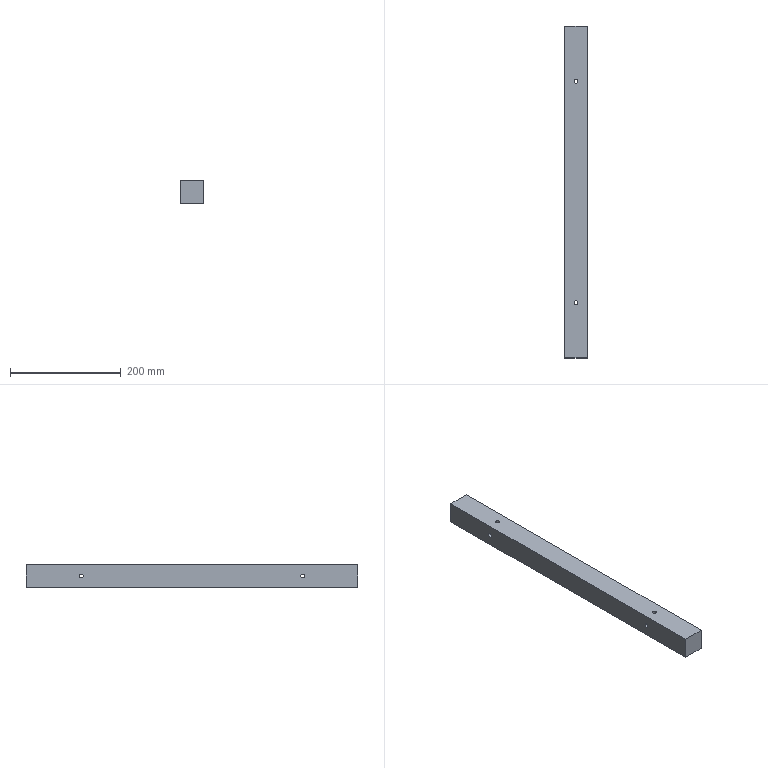Part | NX | features 切除-拉伸3[1] 2 | 1 solid | 22 faces | box 40 x 600 x 40 mm | volume 954300 mm3 | cylinder 16 | plane 6 | commonest cylinder face diameters 7 x16
STEP:
#1=CARTESIAN_POINT('',(-127.,-500.,3.515));
#2=VERTEX_POINT('',#1);
#3=CARTESIAN_POINT('',(-143.5,-500.,3.515));
#4=VERTEX_POINT('',#3);
#5=CARTESIAN_POINT('',(1333.,-500.,3.515));
#6=DIRECTION('',(-1.,0.,0.));
#7=VECTOR('',#6,1000.);
#8=LINE('',#5,#7);
#9=EDGE_CURVE('',#2,#4,#8,.T.);
#10=ORIENTED_EDGE('',*,*,#9,.F.);
#11=CARTESIAN_POINT('',(-127.,-500.,10.515));
#12=VERTEX_POINT('',#11);
#13=CARTESIAN_POINT('',(-127.,-500.,7.015));
#14=DIRECTION('',(1.,0.,0.));
#15=DIRECTION('',(0.,0.,-1.));
#16=AXIS2_PLACEMENT_3D('',#13,#14,#15);
#17=CIRCLE('',#16,3.5);
#18=EDGE_CURVE('',#2,#12,#17,.T.);
#19=ORIENTED_EDGE('',*,*,#18,.T.);
#20=CARTESIAN_POINT('',(-143.5,-500.,10.515));
#21=VERTEX_POINT('',#20);
#22=CARTESIAN_POINT('',(1333.,-500.,10.515));
#23=DIRECTION('',(-1.,0.,0.));
#24=VECTOR('',#23,1000.);
#25=LINE('',#22,#24);
#26=EDGE_CURVE('',#21,#12,#25,.F.);
#27=ORIENTED_EDGE('',*,*,#26,.F.);
#28=CARTESIAN_POINT('',(-147.,-496.5,7.015));
#29=VERTEX_POINT('',#28);
#30=CARTESIAN_POINT('',(-147.,-496.5,7.015));
#31=CARTESIAN_POINT('',(-144.95,-496.5,9.066));
#32=CARTESIAN_POINT('',(-143.5,-497.95,10.515));
#33=CARTESIAN_POINT('',(-143.5,-500.,10.515));
#34=(BOUNDED_CURVE()B_SPLINE_CURVE(3,(#30,#31,#32,#33),.UNSPECIFIED.,.F.,.F.)B_SPLINE_CURVE_WITH_KNOTS((4,4),(4.712,6.283),.UNSPECIFIED.)CURVE()GEOMETRIC_REPRESENTATION_ITEM()RATIONAL_B_SPLINE_CURVE((1.,0.8047,0.8047,1.))REPRESENTATION_ITEM(''));
#35=EDGE_CURVE('',#29,#21,#34,.T.);
#36=ORIENTED_EDGE('',*,*,#35,.F.);
#37=CARTESIAN_POINT('',(-143.5,-500.,3.515));
#38=CARTESIAN_POINT('',(-143.5,-497.95,3.515));
#39=CARTESIAN_POINT('',(-144.95,-496.5,4.965));
#40=CARTESIAN_POINT('',(-147.,-496.5,7.015));
#41=(BOUNDED_CURVE()B_SPLINE_CURVE(3,(#37,#38,#39,#40),.UNSPECIFIED.,.F.,.F.)B_SPLINE_CURVE_WITH_KNOTS((4,4),(3.142,4.712),.UNSPECIFIED.)CURVE()GEOMETRIC_REPRESENTATION_ITEM()RATIONAL_B_SPLINE_CURVE((1.,0.8047,0.8047,1.))REPRESENTATION_ITEM(''));
#42=EDGE_CURVE('',#4,#29,#41,.T.);
#43=ORIENTED_EDGE('',*,*,#42,.F.);
#44=EDGE_LOOP('',(#10,#19,#27,#36,#43));
#45=FACE_BOUND('',#44,.T.);
#46=CARTESIAN_POINT('',(1333.,-500.,7.015));
#47=DIRECTION('',(-1.,0.,0.));
#48=DIRECTION('',(0.,0.,1.));
#49=AXIS2_PLACEMENT_3D('',#46,#47,#48);
#50=CYLINDRICAL_SURFACE('',#49,3.5);
#51=ADVANCED_FACE('',(#45),#50,.F.);
#52=CARTESIAN_POINT('',(-150.5,-500.,3.515));
#53=VERTEX_POINT('',#52);
#54=CARTESIAN_POINT('',(-167.,-500.,3.515));
#55=VERTEX_POINT('',#54);
#56=CARTESIAN_POINT('',(1333.,-500.,3.515));
#57=DIRECTION('',(-1.,0.,0.));
#58=VECTOR('',#57,1000.);
#59=LINE('',#56,#58);
#60=EDGE_CURVE('',#53,#55,#59,.T.);
#61=ORIENTED_EDGE('',*,*,#60,.F.);
#62=CARTESIAN_POINT('',(-147.,-496.5,7.015));
#63=CARTESIAN_POINT('',(-149.05,-496.5,4.965));
#64=CARTESIAN_POINT('',(-150.5,-497.95,3.515));
#65=CARTESIAN_POINT('',(-150.5,-500.,3.515));
#66=(BOUNDED_CURVE()B_SPLINE_CURVE(3,(#62,#63,#64,#65),.UNSPECIFIED.,.F.,.F.)B_SPLINE_CURVE_WITH_KNOTS((4,4),(1.571,3.142),.UNSPECIFIED.)CURVE()GEOMETRIC_REPRESENTATION_ITEM()RATIONAL_B_SPLINE_CURVE((1.,0.8047,0.8047,1.))REPRESENTATION_ITEM(''));
#67=EDGE_CURVE('',#29,#53,#66,.T.);
#68=ORIENTED_EDGE('',*,*,#67,.F.);
#69=CARTESIAN_POINT('',(-150.5,-500.,10.515));
#70=VERTEX_POINT('',#69);
#71=CARTESIAN_POINT('',(-150.5,-500.,10.515));
#72=CARTESIAN_POINT('',(-150.5,-497.95,10.515));
#73=CARTESIAN_POINT('',(-149.05,-496.5,9.066));
#74=CARTESIAN_POINT('',(-147.,-496.5,7.015));
#75=(BOUNDED_CURVE()B_SPLINE_CURVE(3,(#71,#72,#73,#74),.UNSPECIFIED.,.F.,.F.)B_SPLINE_CURVE_WITH_KNOTS((4,4),(0.,1.571),.UNSPECIFIED.)CURVE()GEOMETRIC_REPRESENTATION_ITEM()RATIONAL_B_SPLINE_CURVE((1.,0.8047,0.8047,1.))REPRESENTATION_ITEM(''));
#76=EDGE_CURVE('',#70,#29,#75,.T.);
#77=ORIENTED_EDGE('',*,*,#76,.F.);
#78=CARTESIAN_POINT('',(-167.,-500.,10.515));
#79=VERTEX_POINT('',#78);
#80=CARTESIAN_POINT('',(1333.,-500.,10.515));
#81=DIRECTION('',(-1.,0.,0.));
#82=VECTOR('',#81,1000.);
#83=LINE('',#80,#82);
#84=EDGE_CURVE('',#79,#70,#83,.F.);
#85=ORIENTED_EDGE('',*,*,#84,.F.);
#86=CARTESIAN_POINT('',(-167.,-500.,7.015));
#87=DIRECTION('',(-1.,0.,0.));
#88=DIRECTION('',(0.,0.,1.));
#89=AXIS2_PLACEMENT_3D('',#86,#87,#88);
#90=CIRCLE('',#89,3.5);
#91=EDGE_CURVE('',#79,#55,#90,.T.);
#92=ORIENTED_EDGE('',*,*,#91,.T.);
#93=EDGE_LOOP('',(#61,#68,#77,#85,#92));
#94=FACE_BOUND('',#93,.T.);
#95=CARTESIAN_POINT('',(1333.,-500.,7.015));
#96=DIRECTION('',(-1.,0.,0.));
#97=DIRECTION('',(0.,0.,1.));
#98=AXIS2_PLACEMENT_3D('',#95,#96,#97);
#99=CYLINDRICAL_SURFACE('',#98,3.5);
#100=ADVANCED_FACE('',(#94),#99,.F.);
#101=CARTESIAN_POINT('',(-127.,-100.,3.515));
#102=VERTEX_POINT('',#101);
#103=CARTESIAN_POINT('',(-143.5,-100.,3.515));
#104=VERTEX_POINT('',#103);
#105=CARTESIAN_POINT('',(1333.,-100.,3.515));
#106=DIRECTION('',(-1.,0.,0.));
#107=VECTOR('',#106,1000.);
#108=LINE('',#105,#107);
#109=EDGE_CURVE('',#102,#104,#108,.T.);
#110=ORIENTED_EDGE('',*,*,#109,.F.);
#111=CARTESIAN_POINT('',(-127.,-100.,10.515));
#112=VERTEX_POINT('',#111);
#113=CARTESIAN_POINT('',(-127.,-100.,7.015));
#114=DIRECTION('',(1.,0.,0.));
#115=DIRECTION('',(0.,0.,-1.));
#116=AXIS2_PLACEMENT_3D('',#113,#114,#115);
#117=CIRCLE('',#116,3.5);
#118=EDGE_CURVE('',#102,#112,#117,.T.);
#119=ORIENTED_EDGE('',*,*,#118,.T.);
#120=CARTESIAN_POINT('',(-143.5,-100.,10.515));
#121=VERTEX_POINT('',#120);
#122=CARTESIAN_POINT('',(1333.,-100.,10.515));
#123=DIRECTION('',(-1.,0.,0.));
#124=VECTOR('',#123,1000.);
#125=LINE('',#122,#124);
#126=EDGE_CURVE('',#121,#112,#125,.F.);
#127=ORIENTED_EDGE('',*,*,#126,.F.);
#128=CARTESIAN_POINT('',(-147.,-96.5,7.015));
#129=VERTEX_POINT('',#128);
#130=CARTESIAN_POINT('',(-147.,-96.5,7.015));
#131=CARTESIAN_POINT('',(-144.95,-96.5,9.066));
#132=CARTESIAN_POINT('',(-143.5,-97.95,10.515));
#133=CARTESIAN_POINT('',(-143.5,-100.,10.515));
#134=(BOUNDED_CURVE()B_SPLINE_CURVE(3,(#130,#131,#132,#133),.UNSPECIFIED.,.F.,.F.)B_SPLINE_CURVE_WITH_KNOTS((4,4),(4.712,6.283),.UNSPECIFIED.)CURVE()GEOMETRIC_REPRESENTATION_ITEM()RATIONAL_B_SPLINE_CURVE((1.,0.8047,0.8047,1.))REPRESENTATION_ITEM(''));
#135=EDGE_CURVE('',#129,#121,#134,.T.);
#136=ORIENTED_EDGE('',*,*,#135,.F.);
#137=CARTESIAN_POINT('',(-143.5,-100.,3.515));
#138=CARTESIAN_POINT('',(-143.5,-97.95,3.515));
#139=CARTESIAN_POINT('',(-144.95,-96.5,4.965));
#140=CARTESIAN_POINT('',(-147.,-96.5,7.015));
#141=(BOUNDED_CURVE()B_SPLINE_CURVE(3,(#137,#138,#139,#140),.UNSPECIFIED.,.F.,.F.)B_SPLINE_CURVE_WITH_KNOTS((4,4),(3.142,4.712),.UNSPECIFIED.)CURVE()GEOMETRIC_REPRESENTATION_ITEM()RATIONAL_B_SPLINE_CURVE((1.,0.8047,0.8047,1.))REPRESENTATION_ITEM(''));
#142=EDGE_CURVE('',#104,#129,#141,.T.);
#143=ORIENTED_EDGE('',*,*,#142,.F.);
#144=EDGE_LOOP('',(#110,#119,#127,#136,#143));
#145=FACE_BOUND('',#144,.T.);
#146=CARTESIAN_POINT('',(1333.,-100.,7.015));
#147=DIRECTION('',(-1.,0.,0.));
#148=DIRECTION('',(0.,0.,1.));
#149=AXIS2_PLACEMENT_3D('',#146,#147,#148);
#150=CYLINDRICAL_SURFACE('',#149,3.5);
#151=ADVANCED_FACE('',(#145),#150,.F.);
#152=CARTESIAN_POINT('',(-167.,-100.,3.515));
#153=VERTEX_POINT('',#152);
#154=CARTESIAN_POINT('',(-150.5,-100.,3.515));
#155=VERTEX_POINT('',#154);
#156=CARTESIAN_POINT('',(1333.,-100.,3.515));
#157=DIRECTION('',(-1.,0.,0.));
#158=VECTOR('',#157,1000.);
#159=LINE('',#156,#158);
#160=EDGE_CURVE('',#153,#155,#159,.F.);
#161=ORIENTED_EDGE('',*,*,#160,.T.);
#162=CARTESIAN_POINT('',(-147.,-96.5,7.015));
#163=CARTESIAN_POINT('',(-149.05,-96.5,4.965));
#164=CARTESIAN_POINT('',(-150.5,-97.95,3.515));
#165=CARTESIAN_POINT('',(-150.5,-100.,3.515));
#166=(BOUNDED_CURVE()B_SPLINE_CURVE(3,(#162,#163,#164,#165),.UNSPECIFIED.,.F.,.F.)B_SPLINE_CURVE_WITH_KNOTS((4,4),(1.571,3.142),.UNSPECIFIED.)CURVE()GEOMETRIC_REPRESENTATION_ITEM()RATIONAL_B_SPLINE_CURVE((1.,0.8047,0.8047,1.))REPRESENTATION_ITEM(''));
#167=EDGE_CURVE('',#129,#155,#166,.T.);
#168=ORIENTED_EDGE('',*,*,#167,.F.);
#169=CARTESIAN_POINT('',(-150.5,-100.,10.515));
#170=VERTEX_POINT('',#169);
#171=CARTESIAN_POINT('',(-150.5,-100.,10.515));
#172=CARTESIAN_POINT('',(-150.5,-97.95,10.515));
#173=CARTESIAN_POINT('',(-149.05,-96.5,9.066));
#174=CARTESIAN_POINT('',(-147.,-96.5,7.015));
#175=(BOUNDED_CURVE()B_SPLINE_CURVE(3,(#171,#172,#173,#174),.UNSPECIFIED.,.F.,.F.)B_SPLINE_CURVE_WITH_KNOTS((4,4),(0.,1.571),.UNSPECIFIED.)CURVE()GEOMETRIC_REPRESENTATION_ITEM()RATIONAL_B_SPLINE_CURVE((1.,0.8047,0.8047,1.))REPRESENTATION_ITEM(''));
#176=EDGE_CURVE('',#170,#129,#175,.T.);
#177=ORIENTED_EDGE('',*,*,#176,.F.);
#178=CARTESIAN_POINT('',(-167.,-100.,10.515));
#179=VERTEX_POINT('',#178);
#180=CARTESIAN_POINT('',(1333.,-100.,10.515));
#181=DIRECTION('',(-1.,0.,0.));
#182=VECTOR('',#181,1000.);
#183=LINE('',#180,#182);
#184=EDGE_CURVE('',#170,#179,#183,.T.);
#185=ORIENTED_EDGE('',*,*,#184,.T.);
#186=CARTESIAN_POINT('',(-167.,-100.,7.015));
#187=DIRECTION('',(-1.,0.,0.));
#188=DIRECTION('',(0.,0.,1.));
#189=AXIS2_PLACEMENT_3D('',#186,#187,#188);
#190=CIRCLE('',#189,3.5);
#191=EDGE_CURVE('',#179,#153,#190,.T.);
#192=ORIENTED_EDGE('',*,*,#191,.T.);
#193=EDGE_LOOP('',(#161,#168,#177,#185,#192));
#194=FACE_BOUND('',#193,.T.);
#195=CARTESIAN_POINT('',(1333.,-100.,7.015));
#196=DIRECTION('',(-1.,0.,0.));
#197=DIRECTION('',(0.,0.,1.));
#198=AXIS2_PLACEMENT_3D('',#195,#196,#197);
#199=CYLINDRICAL_SURFACE('',#198,3.5);
#200=ADVANCED_FACE('',(#194),#199,.F.);
#201=CARTESIAN_POINT('',(-150.5,-100.,-12.985));
#202=VERTEX_POINT('',#201);
#203=CARTESIAN_POINT('',(-150.5,-100.,-1372.985));
#204=DIRECTION('',(0.,0.,1.));
#205=VECTOR('',#204,1000.);
#206=LINE('',#203,#205);
#207=EDGE_CURVE('',#202,#155,#206,.T.);
#208=ORIENTED_EDGE('',*,*,#207,.F.);
#209=CARTESIAN_POINT('',(-143.5,-100.,-12.985));
#210=VERTEX_POINT('',#209);
#211=CARTESIAN_POINT('',(-147.,-100.,-12.985));
#212=DIRECTION('',(0.,0.,-1.));
#213=DIRECTION('',(-1.,0.,0.));
#214=AXIS2_PLACEMENT_3D('',#211,#212,#213);
#215=CIRCLE('',#214,3.5);
#216=EDGE_CURVE('',#202,#210,#215,.T.);
#217=ORIENTED_EDGE('',*,*,#216,.T.);
#218=CARTESIAN_POINT('',(-143.5,-100.,-1372.985));
#219=DIRECTION('',(0.,0.,1.));
#220=VECTOR('',#219,1000.);
#221=LINE('',#218,#220);
#222=EDGE_CURVE('',#104,#210,#221,.F.);
#223=ORIENTED_EDGE('',*,*,#222,.F.);
#224=ORIENTED_EDGE('',*,*,#142,.T.);
#225=ORIENTED_EDGE('',*,*,#167,.T.);
#226=EDGE_LOOP('',(#208,#217,#223,#224,#225));
#227=FACE_BOUND('',#226,.T.);
#228=CARTESIAN_POINT('',(-147.,-100.,-1372.985));
#229=DIRECTION('',(0.,0.,1.));
#230=DIRECTION('',(1.,0.,0.));
#231=AXIS2_PLACEMENT_3D('',#228,#229,#230);
#232=CYLINDRICAL_SURFACE('',#231,3.5);
#233=ADVANCED_FACE('',(#227),#232,.F.);
#234=CARTESIAN_POINT('',(-150.5,-500.,-12.985));
#235=VERTEX_POINT('',#234);
#236=CARTESIAN_POINT('',(-150.5,-500.,-1372.985));
#237=DIRECTION('',(0.,0.,1.));
#238=VECTOR('',#237,1000.);
#239=LINE('',#236,#238);
#240=EDGE_CURVE('',#235,#53,#239,.T.);
#241=ORIENTED_EDGE('',*,*,#240,.F.);
#242=CARTESIAN_POINT('',(-143.5,-500.,-12.985));
#243=VERTEX_POINT('',#242);
#244=CARTESIAN_POINT('',(-147.,-500.,-12.985));
#245=DIRECTION('',(0.,0.,-1.));
#246=DIRECTION('',(-1.,0.,0.));
#247=AXIS2_PLACEMENT_3D('',#244,#245,#246);
#248=CIRCLE('',#247,3.5);
#249=EDGE_CURVE('',#235,#243,#248,.T.);
#250=ORIENTED_EDGE('',*,*,#249,.T.);
#251=CARTESIAN_POINT('',(-143.5,-500.,-1372.985));
#252=DIRECTION('',(0.,0.,1.));
#253=VECTOR('',#252,1000.);
#254=LINE('',#251,#253);
#255=EDGE_CURVE('',#4,#243,#254,.F.);
#256=ORIENTED_EDGE('',*,*,#255,.F.);
#257=ORIENTED_EDGE('',*,*,#42,.T.);
#258=ORIENTED_EDGE('',*,*,#67,.T.);
#259=EDGE_LOOP('',(#241,#250,#256,#257,#258));
#260=FACE_BOUND('',#259,.T.);
#261=CARTESIAN_POINT('',(-147.,-500.,-1372.985));
#262=DIRECTION('',(0.,0.,1.));
#263=DIRECTION('',(1.,0.,0.));
#264=AXIS2_PLACEMENT_3D('',#261,#262,#263);
#265=CYLINDRICAL_SURFACE('',#264,3.5);
#266=ADVANCED_FACE('',(#260),#265,.F.);
#267=CARTESIAN_POINT('',(-167.,0.,-12.985));
#268=VERTEX_POINT('',#267);
#269=CARTESIAN_POINT('',(-167.,0.,27.015));
#270=VERTEX_POINT('',#269);
#271=CARTESIAN_POINT('',(-167.,0.,27.015));
#272=DIRECTION('',(0.,0.,1.));
#273=VECTOR('',#272,1000.);
#274=LINE('',#271,#273);
#275=EDGE_CURVE('',#268,#270,#274,.T.);
#276=ORIENTED_EDGE('',*,*,#275,.T.);
#277=CARTESIAN_POINT('',(-127.,0.,27.015));
#278=VERTEX_POINT('',#277);
#279=CARTESIAN_POINT('',(-127.,0.,27.015));
#280=DIRECTION('',(1.,0.,0.));
#281=VECTOR('',#280,1000.);
#282=LINE('',#279,#281);
#283=EDGE_CURVE('',#270,#278,#282,.T.);
#284=ORIENTED_EDGE('',*,*,#283,.T.);
#285=CARTESIAN_POINT('',(-127.,0.,-12.985));
#286=VERTEX_POINT('',#285);
#287=CARTESIAN_POINT('',(-127.,0.,27.015));
#288=DIRECTION('',(0.,0.,-1.));
#289=VECTOR('',#288,1000.);
#290=LINE('',#287,#289);
#291=EDGE_CURVE('',#278,#286,#290,.T.);
#292=ORIENTED_EDGE('',*,*,#291,.T.);
#293=CARTESIAN_POINT('',(-127.,0.,-12.985));
#294=DIRECTION('',(-1.,0.,0.));
#295=VECTOR('',#294,1000.);
#296=LINE('',#293,#295);
#297=EDGE_CURVE('',#286,#268,#296,.T.);
#298=ORIENTED_EDGE('',*,*,#297,.T.);
#299=EDGE_LOOP('',(#276,#284,#292,#298));
#300=FACE_BOUND('',#299,.T.);
#301=CARTESIAN_POINT('',(0.,0.,0.));
#302=DIRECTION('',(0.,1.,0.));
#303=DIRECTION('',(0.,0.,1.));
#304=AXIS2_PLACEMENT_3D('',#301,#302,#303);
#305=PLANE('',#304);
#306=ADVANCED_FACE('',(#300),#305,.T.);
#307=CARTESIAN_POINT('',(-167.,-600.,-12.985));
#308=VERTEX_POINT('',#307);
#309=CARTESIAN_POINT('',(-167.,-600.,27.015));
#310=VERTEX_POINT('',#309);
#311=CARTESIAN_POINT('',(-167.,-600.,27.015));
#312=DIRECTION('',(0.,0.,1.));
#313=VECTOR('',#312,1000.);
#314=LINE('',#311,#313);
#315=EDGE_CURVE('',#308,#310,#314,.T.);
#316=ORIENTED_EDGE('',*,*,#315,.F.);
#317=CARTESIAN_POINT('',(-127.,-600.,-12.985));
#318=VERTEX_POINT('',#317);
#319=CARTESIAN_POINT('',(-127.,-600.,-12.985));
#320=DIRECTION('',(-1.,0.,0.));
#321=VECTOR('',#320,1000.);
#322=LINE('',#319,#321);
#323=EDGE_CURVE('',#318,#308,#322,.T.);
#324=ORIENTED_EDGE('',*,*,#323,.F.);
#325=CARTESIAN_POINT('',(-127.,-600.,27.015));
#326=VERTEX_POINT('',#325);
#327=CARTESIAN_POINT('',(-127.,-600.,27.015));
#328=DIRECTION('',(0.,0.,-1.));
#329=VECTOR('',#328,1000.);
#330=LINE('',#327,#329);
#331=EDGE_CURVE('',#326,#318,#330,.T.);
#332=ORIENTED_EDGE('',*,*,#331,.F.);
#333=CARTESIAN_POINT('',(-127.,-600.,27.015));
#334=DIRECTION('',(1.,0.,0.));
#335=VECTOR('',#334,1000.);
#336=LINE('',#333,#335);
#337=EDGE_CURVE('',#310,#326,#336,.T.);
#338=ORIENTED_EDGE('',*,*,#337,.F.);
#339=EDGE_LOOP('',(#316,#324,#332,#338));
#340=FACE_BOUND('',#339,.T.);
#341=CARTESIAN_POINT('',(0.,-600.,0.));
#342=DIRECTION('',(0.,1.,0.));
#343=DIRECTION('',(0.,0.,1.));
#344=AXIS2_PLACEMENT_3D('',#341,#342,#343);
#345=PLANE('',#344);
#346=ADVANCED_FACE('',(#340),#345,.F.);
#347=ORIENTED_EDGE('',*,*,#283,.F.);
#348=CARTESIAN_POINT('',(-167.,-600.,27.015));
#349=DIRECTION('',(0.,1.,0.));
#350=VECTOR('',#349,1000.);
#351=LINE('',#348,#350);
#352=EDGE_CURVE('',#310,#270,#351,.T.);
#353=ORIENTED_EDGE('',*,*,#352,.F.);
#354=ORIENTED_EDGE('',*,*,#337,.T.);
#355=CARTESIAN_POINT('',(-127.,-600.,27.015));
#356=DIRECTION('',(0.,1.,0.));
#357=VECTOR('',#356,1000.);
#358=LINE('',#355,#357);
#359=EDGE_CURVE('',#326,#278,#358,.T.);
#360=ORIENTED_EDGE('',*,*,#359,.T.);
#361=EDGE_LOOP('',(#347,#353,#354,#360));
#362=FACE_BOUND('',#361,.T.);
#363=CARTESIAN_POINT('',(-143.5,-500.,27.015));
#364=VERTEX_POINT('',#363);
#365=CARTESIAN_POINT('',(-150.5,-500.,27.015));
#366=VERTEX_POINT('',#365);
#367=CARTESIAN_POINT('',(-147.,-500.,27.015));
#368=DIRECTION('',(0.,0.,1.));
#369=DIRECTION('',(1.,0.,0.));
#370=AXIS2_PLACEMENT_3D('',#367,#368,#369);
#371=CIRCLE('',#370,3.5);
#372=EDGE_CURVE('',#364,#366,#371,.T.);
#373=ORIENTED_EDGE('',*,*,#372,.F.);
#374=CARTESIAN_POINT('',(-147.,-500.,27.015));
#375=DIRECTION('',(0.,0.,1.));
#376=DIRECTION('',(1.,0.,0.));
#377=AXIS2_PLACEMENT_3D('',#374,#375,#376);
#378=CIRCLE('',#377,3.5);
#379=EDGE_CURVE('',#366,#364,#378,.T.);
#380=ORIENTED_EDGE('',*,*,#379,.F.);
#381=EDGE_LOOP('',(#373,#380));
#382=FACE_BOUND('',#381,.T.);
#383=CARTESIAN_POINT('',(-143.5,-100.,27.015));
#384=VERTEX_POINT('',#383);
#385=CARTESIAN_POINT('',(-150.5,-100.,27.015));
#386=VERTEX_POINT('',#385);
#387=CARTESIAN_POINT('',(-147.,-100.,27.015));
#388=DIRECTION('',(0.,0.,1.));
#389=DIRECTION('',(1.,0.,0.));
#390=AXIS2_PLACEMENT_3D('',#387,#388,#389);
#391=CIRCLE('',#390,3.5);
#392=EDGE_CURVE('',#384,#386,#391,.T.);
#393=ORIENTED_EDGE('',*,*,#392,.F.);
#394=CARTESIAN_POINT('',(-147.,-100.,27.015));
#395=DIRECTION('',(0.,0.,1.));
#396=DIRECTION('',(1.,0.,0.));
#397=AXIS2_PLACEMENT_3D('',#394,#395,#396);
#398=CIRCLE('',#397,3.5);
#399=EDGE_CURVE('',#386,#384,#398,.T.);
#400=ORIENTED_EDGE('',*,*,#399,.F.);
#401=EDGE_LOOP('',(#393,#400));
#402=FACE_BOUND('',#401,.T.);
#403=CARTESIAN_POINT('',(-127.,-600.,27.015));
#404=DIRECTION('',(0.,0.,1.));
#405=DIRECTION('',(1.,0.,0.));
#406=AXIS2_PLACEMENT_3D('',#403,#404,#405);
#407=PLANE('',#406);
#408=ADVANCED_FACE('',(#362,#382,#402),#407,.T.);
#409=ORIENTED_EDGE('',*,*,#291,.F.);
#410=ORIENTED_EDGE('',*,*,#359,.F.);
#411=ORIENTED_EDGE('',*,*,#331,.T.);
#412=CARTESIAN_POINT('',(-127.,-600.,-12.985));
#413=DIRECTION('',(0.,1.,0.));
#414=VECTOR('',#413,1000.);
#415=LINE('',#412,#414);
#416=EDGE_CURVE('',#318,#286,#415,.T.);
#417=ORIENTED_EDGE('',*,*,#416,.T.);
#418=EDGE_LOOP('',(#409,#410,#411,#417));
#419=FACE_BOUND('',#418,.T.);
#420=CARTESIAN_POINT('',(-127.,-500.,7.015));
#421=DIRECTION('',(1.,0.,0.));
#422=DIRECTION('',(0.,0.,-1.));
#423=AXIS2_PLACEMENT_3D('',#420,#421,#422);
#424=CIRCLE('',#423,3.5);
#425=EDGE_CURVE('',#12,#2,#424,.T.);
#426=ORIENTED_EDGE('',*,*,#425,.F.);
#427=ORIENTED_EDGE('',*,*,#18,.F.);
#428=EDGE_LOOP('',(#426,#427));
#429=FACE_BOUND('',#428,.T.);
#430=CARTESIAN_POINT('',(-127.,-100.,7.015));
#431=DIRECTION('',(1.,0.,0.));
#432=DIRECTION('',(0.,0.,-1.));
#433=AXIS2_PLACEMENT_3D('',#430,#431,#432);
#434=CIRCLE('',#433,3.5);
#435=EDGE_CURVE('',#112,#102,#434,.T.);
#436=ORIENTED_EDGE('',*,*,#435,.F.);
#437=ORIENTED_EDGE('',*,*,#118,.F.);
#438=EDGE_LOOP('',(#436,#437));
#439=FACE_BOUND('',#438,.T.);
#440=CARTESIAN_POINT('',(-127.,-600.,27.015));
#441=DIRECTION('',(1.,0.,0.));
#442=DIRECTION('',(0.,0.,-1.));
#443=AXIS2_PLACEMENT_3D('',#440,#441,#442);
#444=PLANE('',#443);
#445=ADVANCED_FACE('',(#419,#429,#439),#444,.T.);
#446=ORIENTED_EDGE('',*,*,#297,.F.);
#447=ORIENTED_EDGE('',*,*,#416,.F.);
#448=ORIENTED_EDGE('',*,*,#323,.T.);
#449=CARTESIAN_POINT('',(-167.,-600.,-12.985));
#450=DIRECTION('',(0.,1.,0.));
#451=VECTOR('',#450,1000.);
#452=LINE('',#449,#451);
#453=EDGE_CURVE('',#308,#268,#452,.T.);
#454=ORIENTED_EDGE('',*,*,#453,.T.);
#455=EDGE_LOOP('',(#446,#447,#448,#454));
#456=FACE_BOUND('',#455,.T.);
#457=CARTESIAN_POINT('',(-147.,-500.,-12.985));
#458=DIRECTION('',(0.,0.,-1.));
#459=DIRECTION('',(-1.,0.,0.));
#460=AXIS2_PLACEMENT_3D('',#457,#458,#459);
#461=CIRCLE('',#460,3.5);
#462=EDGE_CURVE('',#243,#235,#461,.T.);
#463=ORIENTED_EDGE('',*,*,#462,.F.);
#464=ORIENTED_EDGE('',*,*,#249,.F.);
#465=EDGE_LOOP('',(#463,#464));
#466=FACE_BOUND('',#465,.T.);
#467=CARTESIAN_POINT('',(-147.,-100.,-12.985));
#468=DIRECTION('',(0.,0.,-1.));
#469=DIRECTION('',(-1.,0.,0.));
#470=AXIS2_PLACEMENT_3D('',#467,#468,#469);
#471=CIRCLE('',#470,3.5);
#472=EDGE_CURVE('',#210,#202,#471,.T.);
#473=ORIENTED_EDGE('',*,*,#472,.F.);
#474=ORIENTED_EDGE('',*,*,#216,.F.);
#475=EDGE_LOOP('',(#473,#474));
#476=FACE_BOUND('',#475,.T.);
#477=CARTESIAN_POINT('',(-127.,-600.,-12.985));
#478=DIRECTION('',(0.,0.,-1.));
#479=DIRECTION('',(-1.,0.,0.));
#480=AXIS2_PLACEMENT_3D('',#477,#478,#479);
#481=PLANE('',#480);
#482=ADVANCED_FACE('',(#456,#466,#476),#481,.T.);
#483=ORIENTED_EDGE('',*,*,#275,.F.);
#484=ORIENTED_EDGE('',*,*,#453,.F.);
#485=ORIENTED_EDGE('',*,*,#315,.T.);
#486=ORIENTED_EDGE('',*,*,#352,.T.);
#487=EDGE_LOOP('',(#483,#484,#485,#486));
#488=FACE_BOUND('',#487,.T.);
#489=ORIENTED_EDGE('',*,*,#91,.F.);
#490=CARTESIAN_POINT('',(-167.,-500.,7.015));
#491=DIRECTION('',(-1.,0.,0.));
#492=DIRECTION('',(0.,0.,1.));
#493=AXIS2_PLACEMENT_3D('',#490,#491,#492);
#494=CIRCLE('',#493,3.5);
#495=EDGE_CURVE('',#55,#79,#494,.T.);
#496=ORIENTED_EDGE('',*,*,#495,.F.);
#497=EDGE_LOOP('',(#489,#496));
#498=FACE_BOUND('',#497,.T.);
#499=ORIENTED_EDGE('',*,*,#191,.F.);
#500=CARTESIAN_POINT('',(-167.,-100.,7.015));
#501=DIRECTION('',(-1.,0.,0.));
#502=DIRECTION('',(0.,0.,1.));
#503=AXIS2_PLACEMENT_3D('',#500,#501,#502);
#504=CIRCLE('',#503,3.5);
#505=EDGE_CURVE('',#153,#179,#504,.T.);
#506=ORIENTED_EDGE('',*,*,#505,.F.);
#507=EDGE_LOOP('',(#499,#506));
#508=FACE_BOUND('',#507,.T.);
#509=CARTESIAN_POINT('',(-167.,-600.,27.015));
#510=DIRECTION('',(-1.,0.,0.));
#511=DIRECTION('',(0.,0.,1.));
#512=AXIS2_PLACEMENT_3D('',#509,#510,#511);
#513=PLANE('',#512);
#514=ADVANCED_FACE('',(#488,#498,#508),#513,.T.);
#515=CARTESIAN_POINT('',(-150.5,-100.,-1372.985));
#516=DIRECTION('',(0.,0.,1.));
#517=VECTOR('',#516,1000.);
#518=LINE('',#515,#517);
#519=EDGE_CURVE('',#170,#386,#518,.T.);
#520=ORIENTED_EDGE('',*,*,#519,.F.);
#521=ORIENTED_EDGE('',*,*,#176,.T.);
#522=ORIENTED_EDGE('',*,*,#135,.T.);
#523=CARTESIAN_POINT('',(-143.5,-100.,-1372.985));
#524=DIRECTION('',(0.,0.,1.));
#525=VECTOR('',#524,1000.);
#526=LINE('',#523,#525);
#527=EDGE_CURVE('',#384,#121,#526,.F.);
#528=ORIENTED_EDGE('',*,*,#527,.F.);
#529=ORIENTED_EDGE('',*,*,#392,.T.);
#530=EDGE_LOOP('',(#520,#521,#522,#528,#529));
#531=FACE_BOUND('',#530,.T.);
#532=CARTESIAN_POINT('',(-147.,-100.,-1372.985));
#533=DIRECTION('',(0.,0.,1.));
#534=DIRECTION('',(1.,0.,0.));
#535=AXIS2_PLACEMENT_3D('',#532,#533,#534);
#536=CYLINDRICAL_SURFACE('',#535,3.5);
#537=ADVANCED_FACE('',(#531),#536,.F.);
#538=CARTESIAN_POINT('',(-150.5,-500.,-1372.985));
#539=DIRECTION('',(0.,0.,1.));
#540=VECTOR('',#539,1000.);
#541=LINE('',#538,#540);
#542=EDGE_CURVE('',#70,#366,#541,.T.);
#543=ORIENTED_EDGE('',*,*,#542,.F.);
#544=ORIENTED_EDGE('',*,*,#76,.T.);
#545=ORIENTED_EDGE('',*,*,#35,.T.);
#546=CARTESIAN_POINT('',(-143.5,-500.,-1372.985));
#547=DIRECTION('',(0.,0.,1.));
#548=VECTOR('',#547,1000.);
#549=LINE('',#546,#548);
#550=EDGE_CURVE('',#364,#21,#549,.F.);
#551=ORIENTED_EDGE('',*,*,#550,.F.);
#552=ORIENTED_EDGE('',*,*,#372,.T.);
#553=EDGE_LOOP('',(#543,#544,#545,#551,#552));
#554=FACE_BOUND('',#553,.T.);
#555=CARTESIAN_POINT('',(-147.,-500.,-1372.985));
#556=DIRECTION('',(0.,0.,1.));
#557=DIRECTION('',(1.,0.,0.));
#558=AXIS2_PLACEMENT_3D('',#555,#556,#557);
#559=CYLINDRICAL_SURFACE('',#558,3.5);
#560=ADVANCED_FACE('',(#554),#559,.F.);
#561=CARTESIAN_POINT('',(-147.,-503.5,7.015));
#562=VERTEX_POINT('',#561);
#563=CARTESIAN_POINT('',(-147.,-503.5,7.015));
#564=CARTESIAN_POINT('',(-149.05,-503.5,9.066));
#565=CARTESIAN_POINT('',(-150.5,-502.05,10.515));
#566=CARTESIAN_POINT('',(-150.5,-500.,10.515));
#567=(BOUNDED_CURVE()B_SPLINE_CURVE(3,(#563,#564,#565,#566),.UNSPECIFIED.,.F.,.F.)B_SPLINE_CURVE_WITH_KNOTS((4,4),(4.712,6.283),.UNSPECIFIED.)CURVE()GEOMETRIC_REPRESENTATION_ITEM()RATIONAL_B_SPLINE_CURVE((1.,0.8047,0.8047,1.))REPRESENTATION_ITEM(''));
#568=EDGE_CURVE('',#562,#70,#567,.T.);
#569=ORIENTED_EDGE('',*,*,#568,.T.);
#570=ORIENTED_EDGE('',*,*,#542,.T.);
#571=ORIENTED_EDGE('',*,*,#379,.T.);
#572=ORIENTED_EDGE('',*,*,#550,.T.);
#573=CARTESIAN_POINT('',(-143.5,-500.,10.515));
#574=CARTESIAN_POINT('',(-143.5,-502.05,10.515));
#575=CARTESIAN_POINT('',(-144.95,-503.5,9.066));
#576=CARTESIAN_POINT('',(-147.,-503.5,7.015));
#577=(BOUNDED_CURVE()B_SPLINE_CURVE(3,(#573,#574,#575,#576),.UNSPECIFIED.,.F.,.F.)B_SPLINE_CURVE_WITH_KNOTS((4,4),(0.,1.571),.UNSPECIFIED.)CURVE()GEOMETRIC_REPRESENTATION_ITEM()RATIONAL_B_SPLINE_CURVE((1.,0.8047,0.8047,1.))REPRESENTATION_ITEM(''));
#578=EDGE_CURVE('',#21,#562,#577,.T.);
#579=ORIENTED_EDGE('',*,*,#578,.T.);
#580=EDGE_LOOP('',(#569,#570,#571,#572,#579));
#581=FACE_BOUND('',#580,.T.);
#582=CARTESIAN_POINT('',(-147.,-500.,-1372.985));
#583=DIRECTION('',(0.,0.,1.));
#584=DIRECTION('',(1.,0.,0.));
#585=AXIS2_PLACEMENT_3D('',#582,#583,#584);
#586=CYLINDRICAL_SURFACE('',#585,3.5);
#587=ADVANCED_FACE('',(#581),#586,.F.);
#588=CARTESIAN_POINT('',(-147.,-103.5,7.015));
#589=VERTEX_POINT('',#588);
#590=CARTESIAN_POINT('',(-147.,-103.5,7.015));
#591=CARTESIAN_POINT('',(-149.05,-103.5,9.066));
#592=CARTESIAN_POINT('',(-150.5,-102.05,10.515));
#593=CARTESIAN_POINT('',(-150.5,-100.,10.515));
#594=(BOUNDED_CURVE()B_SPLINE_CURVE(3,(#590,#591,#592,#593),.UNSPECIFIED.,.F.,.F.)B_SPLINE_CURVE_WITH_KNOTS((4,4),(4.712,6.283),.UNSPECIFIED.)CURVE()GEOMETRIC_REPRESENTATION_ITEM()RATIONAL_B_SPLINE_CURVE((1.,0.8047,0.8047,1.))REPRESENTATION_ITEM(''));
#595=EDGE_CURVE('',#589,#170,#594,.T.);
#596=ORIENTED_EDGE('',*,*,#595,.T.);
#597=ORIENTED_EDGE('',*,*,#519,.T.);
#598=ORIENTED_EDGE('',*,*,#399,.T.);
#599=ORIENTED_EDGE('',*,*,#527,.T.);
#600=CARTESIAN_POINT('',(-143.5,-100.,10.515));
#601=CARTESIAN_POINT('',(-143.5,-102.05,10.515));
#602=CARTESIAN_POINT('',(-144.95,-103.5,9.066));
#603=CARTESIAN_POINT('',(-147.,-103.5,7.015));
#604=(BOUNDED_CURVE()B_SPLINE_CURVE(3,(#600,#601,#602,#603),.UNSPECIFIED.,.F.,.F.)B_SPLINE_CURVE_WITH_KNOTS((4,4),(0.,1.571),.UNSPECIFIED.)CURVE()GEOMETRIC_REPRESENTATION_ITEM()RATIONAL_B_SPLINE_CURVE((1.,0.8047,0.8047,1.))REPRESENTATION_ITEM(''));
#605=EDGE_CURVE('',#121,#589,#604,.T.);
#606=ORIENTED_EDGE('',*,*,#605,.T.);
#607=EDGE_LOOP('',(#596,#597,#598,#599,#606));
#608=FACE_BOUND('',#607,.T.);
#609=CARTESIAN_POINT('',(-147.,-100.,-1372.985));
#610=DIRECTION('',(0.,0.,1.));
#611=DIRECTION('',(1.,0.,0.));
#612=AXIS2_PLACEMENT_3D('',#609,#610,#611);
#613=CYLINDRICAL_SURFACE('',#612,3.5);
#614=ADVANCED_FACE('',(#608),#613,.F.);
#615=ORIENTED_EDGE('',*,*,#462,.T.);
#616=ORIENTED_EDGE('',*,*,#240,.T.);
#617=CARTESIAN_POINT('',(-150.5,-500.,3.515));
#618=CARTESIAN_POINT('',(-150.5,-502.05,3.515));
#619=CARTESIAN_POINT('',(-149.05,-503.5,4.965));
#620=CARTESIAN_POINT('',(-147.,-503.5,7.015));
#621=(BOUNDED_CURVE()B_SPLINE_CURVE(3,(#617,#618,#619,#620),.UNSPECIFIED.,.F.,.F.)B_SPLINE_CURVE_WITH_KNOTS((4,4),(3.142,4.712),.UNSPECIFIED.)CURVE()GEOMETRIC_REPRESENTATION_ITEM()RATIONAL_B_SPLINE_CURVE((1.,0.8047,0.8047,1.))REPRESENTATION_ITEM(''));
#622=EDGE_CURVE('',#53,#562,#621,.T.);
#623=ORIENTED_EDGE('',*,*,#622,.T.);
#624=CARTESIAN_POINT('',(-147.,-503.5,7.015));
#625=CARTESIAN_POINT('',(-144.95,-503.5,4.965));
#626=CARTESIAN_POINT('',(-143.5,-502.05,3.515));
#627=CARTESIAN_POINT('',(-143.5,-500.,3.515));
#628=(BOUNDED_CURVE()B_SPLINE_CURVE(3,(#624,#625,#626,#627),.UNSPECIFIED.,.F.,.F.)B_SPLINE_CURVE_WITH_KNOTS((4,4),(1.571,3.142),.UNSPECIFIED.)CURVE()GEOMETRIC_REPRESENTATION_ITEM()RATIONAL_B_SPLINE_CURVE((1.,0.8047,0.8047,1.))REPRESENTATION_ITEM(''));
#629=EDGE_CURVE('',#562,#4,#628,.T.);
#630=ORIENTED_EDGE('',*,*,#629,.T.);
#631=ORIENTED_EDGE('',*,*,#255,.T.);
#632=EDGE_LOOP('',(#615,#616,#623,#630,#631));
#633=FACE_BOUND('',#632,.T.);
#634=CARTESIAN_POINT('',(-147.,-500.,-1372.985));
#635=DIRECTION('',(0.,0.,1.));
#636=DIRECTION('',(1.,0.,0.));
#637=AXIS2_PLACEMENT_3D('',#634,#635,#636);
#638=CYLINDRICAL_SURFACE('',#637,3.5);
#639=ADVANCED_FACE('',(#633),#638,.F.);
#640=ORIENTED_EDGE('',*,*,#472,.T.);
#641=ORIENTED_EDGE('',*,*,#207,.T.);
#642=CARTESIAN_POINT('',(-150.5,-100.,3.515));
#643=CARTESIAN_POINT('',(-150.5,-102.05,3.515));
#644=CARTESIAN_POINT('',(-149.05,-103.5,4.965));
#645=CARTESIAN_POINT('',(-147.,-103.5,7.015));
#646=(BOUNDED_CURVE()B_SPLINE_CURVE(3,(#642,#643,#644,#645),.UNSPECIFIED.,.F.,.F.)B_SPLINE_CURVE_WITH_KNOTS((4,4),(3.142,4.712),.UNSPECIFIED.)CURVE()GEOMETRIC_REPRESENTATION_ITEM()RATIONAL_B_SPLINE_CURVE((1.,0.8047,0.8047,1.))REPRESENTATION_ITEM(''));
#647=EDGE_CURVE('',#155,#589,#646,.T.);
#648=ORIENTED_EDGE('',*,*,#647,.T.);
#649=CARTESIAN_POINT('',(-147.,-103.5,7.015));
#650=CARTESIAN_POINT('',(-144.95,-103.5,4.965));
#651=CARTESIAN_POINT('',(-143.5,-102.05,3.515));
#652=CARTESIAN_POINT('',(-143.5,-100.,3.515));
#653=(BOUNDED_CURVE()B_SPLINE_CURVE(3,(#649,#650,#651,#652),.UNSPECIFIED.,.F.,.F.)B_SPLINE_CURVE_WITH_KNOTS((4,4),(1.571,3.142),.UNSPECIFIED.)CURVE()GEOMETRIC_REPRESENTATION_ITEM()RATIONAL_B_SPLINE_CURVE((1.,0.8047,0.8047,1.))REPRESENTATION_ITEM(''));
#654=EDGE_CURVE('',#589,#104,#653,.T.);
#655=ORIENTED_EDGE('',*,*,#654,.T.);
#656=ORIENTED_EDGE('',*,*,#222,.T.);
#657=EDGE_LOOP('',(#640,#641,#648,#655,#656));
#658=FACE_BOUND('',#657,.T.);
#659=CARTESIAN_POINT('',(-147.,-100.,-1372.985));
#660=DIRECTION('',(0.,0.,1.));
#661=DIRECTION('',(1.,0.,0.));
#662=AXIS2_PLACEMENT_3D('',#659,#660,#661);
#663=CYLINDRICAL_SURFACE('',#662,3.5);
#664=ADVANCED_FACE('',(#658),#663,.F.);
#665=ORIENTED_EDGE('',*,*,#647,.F.);
#666=ORIENTED_EDGE('',*,*,#160,.F.);
#667=ORIENTED_EDGE('',*,*,#505,.T.);
#668=ORIENTED_EDGE('',*,*,#184,.F.);
#669=ORIENTED_EDGE('',*,*,#595,.F.);
#670=EDGE_LOOP('',(#665,#666,#667,#668,#669));
#671=FACE_BOUND('',#670,.T.);
#672=CARTESIAN_POINT('',(1333.,-100.,7.015));
#673=DIRECTION('',(-1.,0.,0.));
#674=DIRECTION('',(0.,0.,1.));
#675=AXIS2_PLACEMENT_3D('',#672,#673,#674);
#676=CYLINDRICAL_SURFACE('',#675,3.5);
#677=ADVANCED_FACE('',(#671),#676,.F.);
#678=ORIENTED_EDGE('',*,*,#435,.T.);
#679=ORIENTED_EDGE('',*,*,#109,.T.);
#680=ORIENTED_EDGE('',*,*,#654,.F.);
#681=ORIENTED_EDGE('',*,*,#605,.F.);
#682=ORIENTED_EDGE('',*,*,#126,.T.);
#683=EDGE_LOOP('',(#678,#679,#680,#681,#682));
#684=FACE_BOUND('',#683,.T.);
#685=CARTESIAN_POINT('',(1333.,-100.,7.015));
#686=DIRECTION('',(-1.,0.,0.));
#687=DIRECTION('',(0.,0.,1.));
#688=AXIS2_PLACEMENT_3D('',#685,#686,#687);
#689=CYLINDRICAL_SURFACE('',#688,3.5);
#690=ADVANCED_FACE('',(#684),#689,.F.);
#691=ORIENTED_EDGE('',*,*,#622,.F.);
#692=ORIENTED_EDGE('',*,*,#60,.T.);
#693=ORIENTED_EDGE('',*,*,#495,.T.);
#694=ORIENTED_EDGE('',*,*,#84,.T.);
#695=ORIENTED_EDGE('',*,*,#568,.F.);
#696=EDGE_LOOP('',(#691,#692,#693,#694,#695));
#697=FACE_BOUND('',#696,.T.);
#698=CARTESIAN_POINT('',(1333.,-500.,7.015));
#699=DIRECTION('',(-1.,0.,0.));
#700=DIRECTION('',(0.,0.,1.));
#701=AXIS2_PLACEMENT_3D('',#698,#699,#700);
#702=CYLINDRICAL_SURFACE('',#701,3.5);
#703=ADVANCED_FACE('',(#697),#702,.F.);
#704=ORIENTED_EDGE('',*,*,#425,.T.);
#705=ORIENTED_EDGE('',*,*,#9,.T.);
#706=ORIENTED_EDGE('',*,*,#629,.F.);
#707=ORIENTED_EDGE('',*,*,#578,.F.);
#708=ORIENTED_EDGE('',*,*,#26,.T.);
#709=EDGE_LOOP('',(#704,#705,#706,#707,#708));
#710=FACE_BOUND('',#709,.T.);
#711=CARTESIAN_POINT('',(1333.,-500.,7.015));
#712=DIRECTION('',(-1.,0.,0.));
#713=DIRECTION('',(0.,0.,1.));
#714=AXIS2_PLACEMENT_3D('',#711,#712,#713);
#715=CYLINDRICAL_SURFACE('',#714,3.5);
#716=ADVANCED_FACE('',(#710),#715,.F.);
#717=CLOSED_SHELL('',(#51,#100,#151,#200,#233,#266,#306,#346,#408,#445,#482,#514,#537,#560,#587,#614,#639,#664,#677,#690,#703,#716));
#718=MANIFOLD_SOLID_BREP('',#717);
#719=(LENGTH_UNIT()NAMED_UNIT(*)SI_UNIT(.MILLI.,.METRE.));
#720=UNCERTAINTY_MEASURE_WITH_UNIT(LENGTH_MEASURE(0.00001),#719,'','');
#721=(NAMED_UNIT(*)PLANE_ANGLE_UNIT()SI_UNIT($,.RADIAN.));
#722=(NAMED_UNIT(*)SI_UNIT($,.STERADIAN.)SOLID_ANGLE_UNIT());
#723=(GEOMETRIC_REPRESENTATION_CONTEXT(3)GLOBAL_UNCERTAINTY_ASSIGNED_CONTEXT((#720))GLOBAL_UNIT_ASSIGNED_CONTEXT((#719,#721,#722))REPRESENTATION_CONTEXT('',''));
#724=ADVANCED_BREP_SHAPE_REPRESENTATION('',(#718),#723);